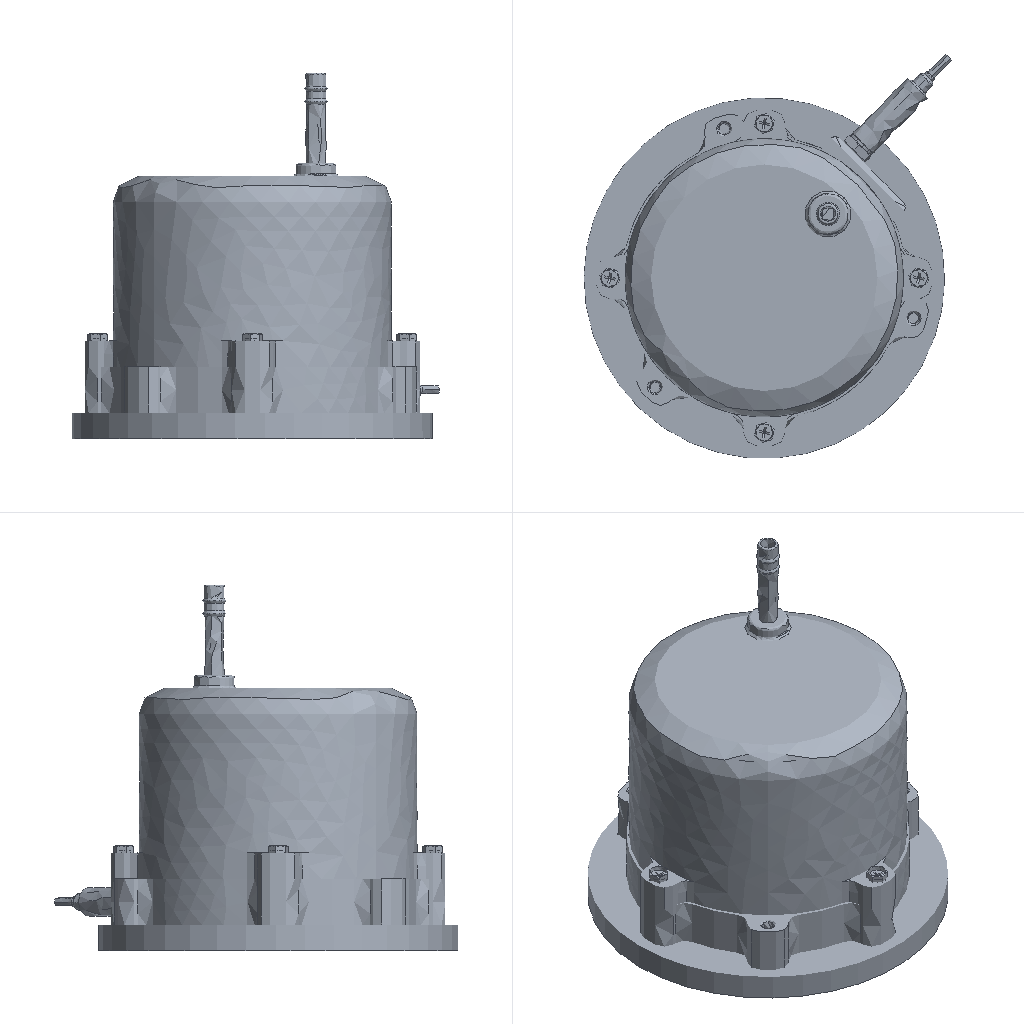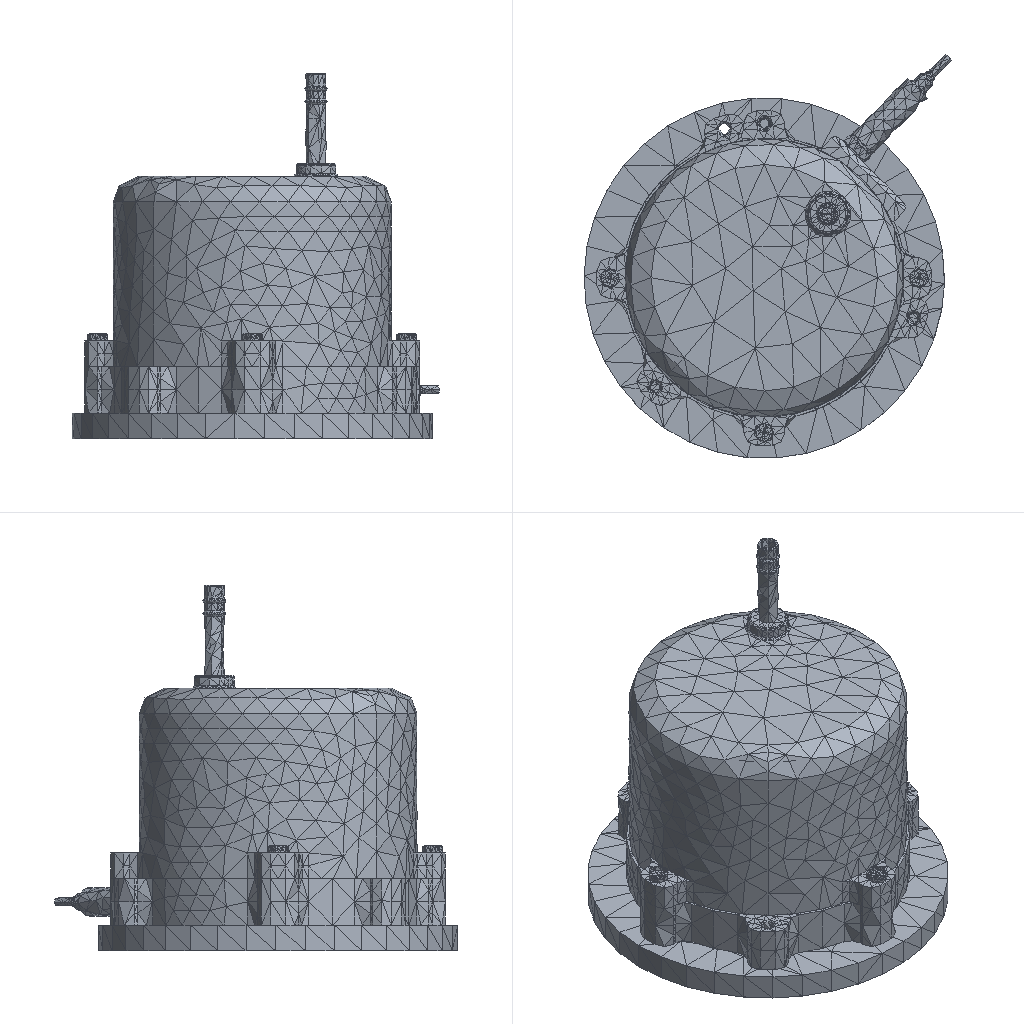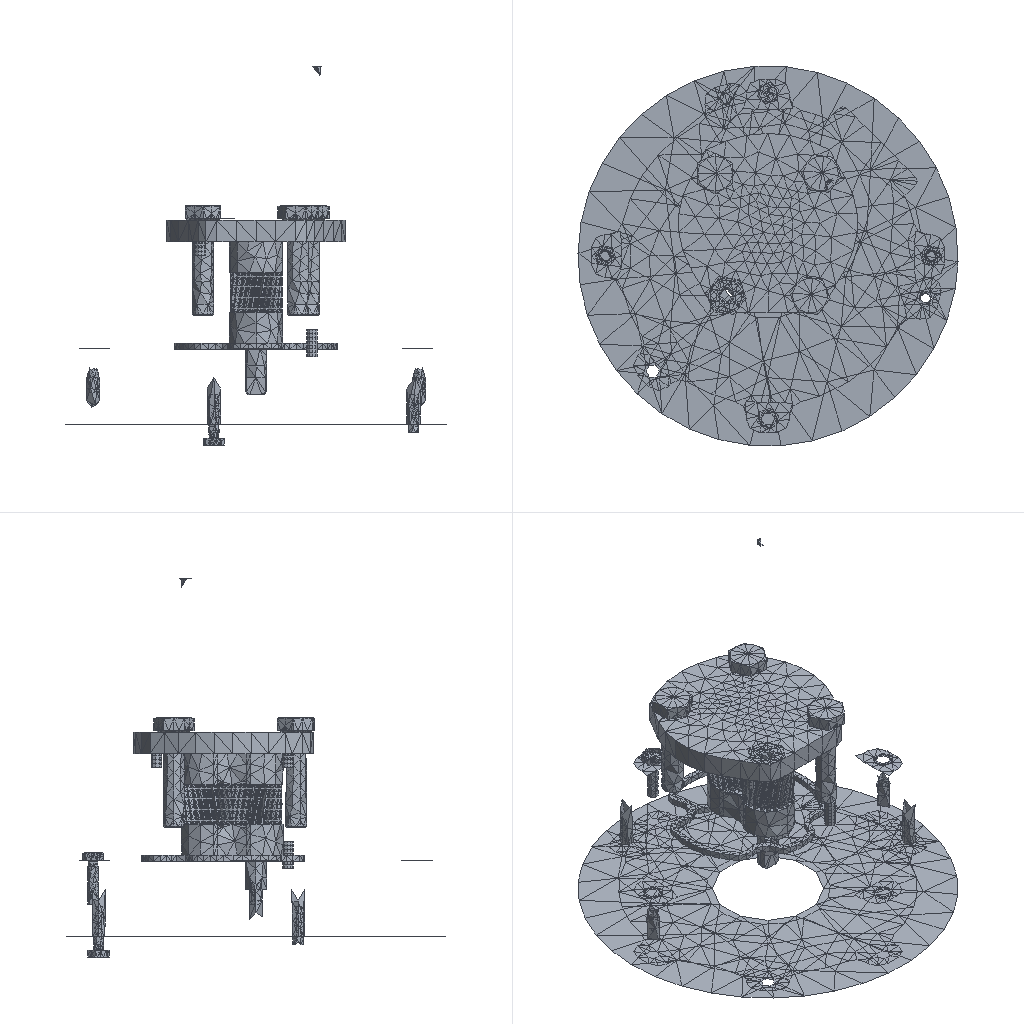Simulation study | ansys workbench
Set-up summary:
category,name,step,type,value,unit,region
solver,ansys_workbench
units,mm-N-s-tonne (MPa),,stated,"/units,MPA"
analysis,deck-1/LS1,,modal,method=lanb; n_modes=6
load_step,deck-1/LS1,deck-1/LS1,modal
analysis,deck-2/LS1,,modal,restart=True
load_step,deck-2/LS1,deck-2/LS1,modal
analysis,deck-2/LS1,,harm
load_step,deck-2/LS1,deck-2/LS1,harm,nsubst=4
load_step,deck-2/LS1,deck-2/LS1,harm
mesh,deck-1.dat,,nodes,110134
mesh,deck-1.dat,,elements,78461
element_type,SOLID187,,,56857,,deck-1.dat
element_type,TARGE170,,,10422,,deck-1.dat
element_type,CONTA174,,,10422,,deck-1.dat
element_type,SOLID186,,,760,,deck-1.dat
mesh,deck-2.dat,,nodes,0
mesh,deck-2.dat,,elements,84
mesh,deck-2.dat,,note,"restart analysis: no node block, runs on the mesh of the upstream system's deck"
element_type,SURF154,,,84,,deck-2.dat
material,Structural Steel,,E,200000,tonne s^-2 mm^-1
material,Structural Steel,,nu,0.3
material,Structural Steel,,density,7.85e-09,tonne mm^-3
material,Structural Steel,,conductivity,60.5,tonne mm s^-3 C^-1
material,Structural Steel,,specific_heat,4.34e+08,mm^2 s^-2 C^-1
material,Structural Steel,,cte,1.2e-05,C^-1
material,Structural Steel,,permeability,10000
material,Structural Steel,,resistivity,0.00017,ohm mm
load,Define Force Using Surface Effect Elements,deck-2/LS1,surface-effect pres face 3,1,,SURF154 #137
bc,Fixed Supports,deck-1/model,fixed,[dofs=ALL],,_FIXEDSU
contact,Contact Region,,bonded (always),element=CONTA174
contact,Contact Region 3,,bonded (always),element=CONTA174
contact,Contact Region 4,,bonded (always),element=CONTA174
contact,Contact Region 5,,bonded (always),element=CONTA174
contact,Contact Region 6,,bonded (always),element=CONTA174
contact,Contact Region 7,,bonded (always),element=CONTA174
contact,Contact Region 9,,bonded (always),element=CONTA174
contact,Contact Region 10,,bonded (always),element=CONTA174
contact,Contact Region 11,,bonded (always),element=CONTA174
contact,Contact Region 12,,bonded (always),element=CONTA174
contact,Contact Region 13,,bonded (always),element=CONTA174
contact,Contact Region 14,,bonded (always),element=CONTA174
contact,Contact Region 15,,bonded (always),element=CONTA174
contact,Contact Region 16,,bonded (always),element=CONTA174
contact,Contact Region 17,,bonded (always),element=CONTA174
contact,Contact Region 18,,bonded (always),element=CONTA174
contact,Contact Region 19,,bonded (always),element=CONTA174
contact,Contact Region 20,,bonded (always),element=CONTA174
contact,Contact Region 21,,bonded (always),element=CONTA174
contact,Contact Region 22,,bonded (always),element=CONTA174
contact,Contact Region 23,,bonded (always),element=CONTA174
contact,Contact Region 24,,bonded (always),element=CONTA174
contact,Contact Region 25,,bonded (always),element=CONTA174
contact,Contact Region 27,,bonded (always),element=CONTA174
contact,Contact Region 28,,bonded (always),element=CONTA174
contact,Contact Region 30,,bonded (always),element=CONTA174
contact,Contact Region 31,,bonded (always),element=CONTA174
contact,Contact Region 32,,bonded (always),element=CONTA174
contact,Contact Region 33,,bonded (always),element=CONTA174
contact,Contact Region 34,,bonded (always),element=CONTA174
contact,Contact Region 35,,bonded (always),element=CONTA174
contact,Contact Region 36,,bonded (always),element=CONTA174
contact,Contact Region 37,,bonded (always),element=CONTA174
contact,Contact Region 39,,bonded (always),element=CONTA174
contact,Contact Region 40,,bonded (always),element=CONTA174
contact,Contact Region 48,,bonded (always),element=CONTA174
contact,Contact Region 49,,bonded (always),element=CONTA174
contact,Contact Region 50,,bonded (always),element=CONTA174
contact,Contact Region 51,,bonded (always),element=CONTA174
contact,Contact Region 52,,bonded (always),element=CONTA174
contact,Contact Region 53,,bonded (always),element=CONTA174
contact,Contact Region 54,,bonded (always),element=CONTA174
contact,Contact Region 55,,bonded (always),element=CONTA174
contact,Contact Region 56,,bonded (always),element=CONTA174
contact,Contact Region 57,,bonded (always),element=CONTA174
contact,Contact Region 58,,bonded (always),element=CONTA174
contact,Contact Region 59,,bonded (always),element=CONTA174
contact,Contact Region 60,,bonded (always),element=CONTA174
contact,Contact Region 61,,bonded (always),element=CONTA174
contact,Contact Region 62,,bonded (always),element=CONTA174
contact,Contact Region 63,,bonded (always),element=CONTA174
contact,Contact Region 64,,bonded (always),element=CONTA174
contact,Contact Region 65,,bonded (always),element=CONTA174
named_set,_CM332_FIXEDSU,,node,333
named_set,_FIXEDSU,,node,333
Results summary:
result,analyses[0].index,,,1
result,analyses[0].system,,,SYS
result,analyses[0].deck,,,deck-1.dat
result,analyses[0].solve_status,,,completed
result,analyses[0].analysis_type,,,modal
result,analyses[0].physics,,,mechanical
result,analyses[0].unit_system,,,"NMM: mm, ton, N, s, mV, mA, degC"
result,analyses[0].n_sets,,,6
result,analyses[0].modal_frequencies_hz[1],,,1709.32
result,analyses[0].modal_frequencies_hz[2],,,2405.05
result,analyses[0].modal_frequencies_hz[3],,,2803.56
result,analyses[0].modal_frequencies_hz[4],,,2880.07
result,analyses[0].modal_frequencies_hz[5],,,3651.88
result,analyses[0].modal_frequencies_hz[6],,,3798.22
result,analyses[1].index,,,2
result,analyses[1].system,,,SYS-1
result,analyses[1].deck,,,deck-2.dat
result,analyses[1].solve_status,,,completed
result,analyses[1].analysis_type,,,MSUP
result,analyses[1].physics,,,mechanical
result,analyses[1].unit_system,,,"NMM: mm, ton, N, s, mV, mA, degC"
result,analyses[1].n_sets,,,2
result,analyses[1].load_steps[0].set,set=2,,2
result,analyses[1].load_steps[0].time_or_freq,set=2,,480
result,analyses[1].load_steps[0].max_displacement_magnitude,set=2,,0.0004847
result,analyses[1].load_steps[0].max_von_mises_nodal,set=2,,0.2607
result,analyses[1].load_steps[0].reaction_force_sum_xyz[1],set=2,,0.6675
result,analyses[1].load_steps[0].reaction_force_sum_xyz[2],set=2,,0.6711
result,analyses[1].load_steps[0].reaction_force_sum_xyz[3],set=2,,7.805